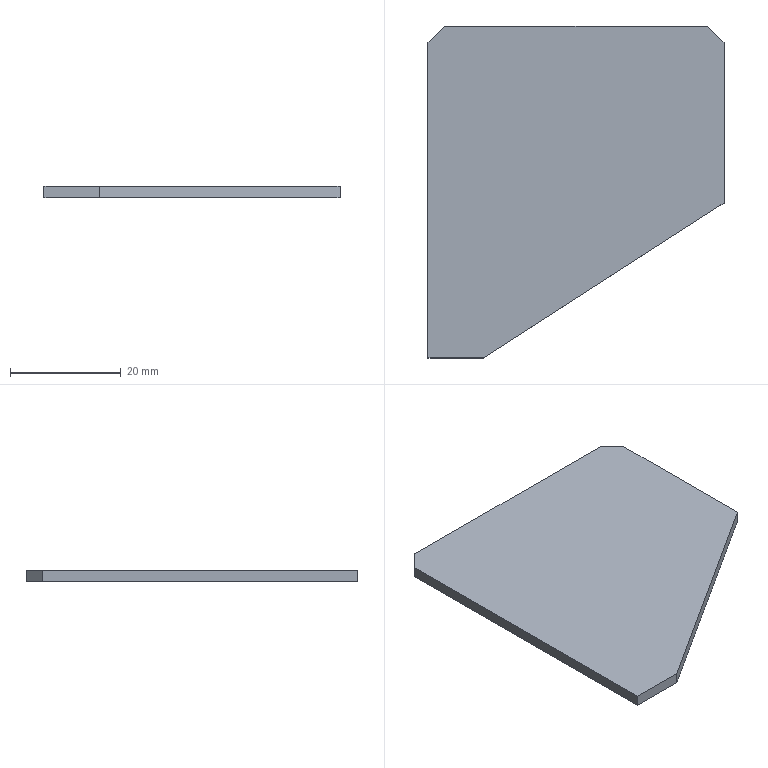Part | SolidWorks | features Chamfer 1, Extrusion 1 | 1 solid | 9 faces | box 53.5 x 60 x 2 mm | volume 5184 mm3 | plane 9
STEP:
#1=CARTESIAN_POINT('',(0.,-3.,2.));
#2=VERTEX_POINT('',#1);
#3=CARTESIAN_POINT('',(0.,-60.,2.));
#4=VERTEX_POINT('',#3);
#5=CARTESIAN_POINT('',(0.,-60.,2.));
#6=DIRECTION('',(0.,-1.,0.));
#7=VECTOR('',#6,1000.);
#8=LINE('',#5,#7);
#9=EDGE_CURVE('',#2,#4,#8,.T.);
#10=ORIENTED_EDGE('',*,*,#9,.F.);
#11=CARTESIAN_POINT('',(0.,-3.,0.));
#12=VERTEX_POINT('',#11);
#13=CARTESIAN_POINT('',(0.,-3.,2.));
#14=DIRECTION('',(0.,0.,-1.));
#15=VECTOR('',#14,1000.);
#16=LINE('',#13,#15);
#17=EDGE_CURVE('',#2,#12,#16,.T.);
#18=ORIENTED_EDGE('',*,*,#17,.T.);
#19=CARTESIAN_POINT('',(0.,-60.,0.));
#20=VERTEX_POINT('',#19);
#21=CARTESIAN_POINT('',(0.,-60.,0.));
#22=DIRECTION('',(0.,-1.,0.));
#23=VECTOR('',#22,1000.);
#24=LINE('',#21,#23);
#25=EDGE_CURVE('',#12,#20,#24,.T.);
#26=ORIENTED_EDGE('',*,*,#25,.T.);
#27=CARTESIAN_POINT('',(0.,-60.,2.));
#28=DIRECTION('',(0.,0.,-1.));
#29=VECTOR('',#28,1000.);
#30=LINE('',#27,#29);
#31=EDGE_CURVE('',#4,#20,#30,.T.);
#32=ORIENTED_EDGE('',*,*,#31,.F.);
#33=EDGE_LOOP('',(#10,#18,#26,#32));
#34=FACE_OUTER_BOUND('',#33,.T.);
#35=CARTESIAN_POINT('',(0.,-60.,2.));
#36=DIRECTION('',(1.,0.,0.));
#37=DIRECTION('',(0.,0.,-1.));
#38=AXIS2_PLACEMENT_3D('',#35,#36,#37);
#39=PLANE('',#38);
#40=ADVANCED_FACE('',(#34),#39,.F.);
#41=CARTESIAN_POINT('',(10.,-60.,0.));
#42=VERTEX_POINT('',#41);
#43=CARTESIAN_POINT('',(10.,-60.,0.));
#44=DIRECTION('',(1.,0.,0.));
#45=VECTOR('',#44,1000.);
#46=LINE('',#43,#45);
#47=EDGE_CURVE('',#20,#42,#46,.T.);
#48=ORIENTED_EDGE('',*,*,#47,.T.);
#49=CARTESIAN_POINT('',(10.,-60.,2.));
#50=VERTEX_POINT('',#49);
#51=CARTESIAN_POINT('',(10.,-60.,2.));
#52=DIRECTION('',(0.,0.,-1.));
#53=VECTOR('',#52,1000.);
#54=LINE('',#51,#53);
#55=EDGE_CURVE('',#50,#42,#54,.T.);
#56=ORIENTED_EDGE('',*,*,#55,.F.);
#57=CARTESIAN_POINT('',(10.,-60.,2.));
#58=DIRECTION('',(1.,0.,0.));
#59=VECTOR('',#58,1000.);
#60=LINE('',#57,#59);
#61=EDGE_CURVE('',#4,#50,#60,.T.);
#62=ORIENTED_EDGE('',*,*,#61,.F.);
#63=ORIENTED_EDGE('',*,*,#31,.T.);
#64=EDGE_LOOP('',(#48,#56,#62,#63));
#65=FACE_OUTER_BOUND('',#64,.T.);
#66=CARTESIAN_POINT('',(10.,-60.,2.));
#67=DIRECTION('',(0.,1.,0.));
#68=DIRECTION('',(0.,0.,1.));
#69=AXIS2_PLACEMENT_3D('',#66,#67,#68);
#70=PLANE('',#69);
#71=ADVANCED_FACE('',(#65),#70,.F.);
#72=CARTESIAN_POINT('',(53.5,-32.,0.));
#73=VERTEX_POINT('',#72);
#74=CARTESIAN_POINT('',(53.5,-32.,0.));
#75=DIRECTION('',(0.8409,0.5412,0.));
#76=VECTOR('',#75,1000.);
#77=LINE('',#74,#76);
#78=EDGE_CURVE('',#42,#73,#77,.T.);
#79=ORIENTED_EDGE('',*,*,#78,.T.);
#80=CARTESIAN_POINT('',(53.5,-32.,2.));
#81=VERTEX_POINT('',#80);
#82=CARTESIAN_POINT('',(53.5,-32.,2.));
#83=DIRECTION('',(0.,0.,-1.));
#84=VECTOR('',#83,1000.);
#85=LINE('',#82,#84);
#86=EDGE_CURVE('',#81,#73,#85,.T.);
#87=ORIENTED_EDGE('',*,*,#86,.F.);
#88=CARTESIAN_POINT('',(53.5,-32.,2.));
#89=DIRECTION('',(0.8409,0.5412,0.));
#90=VECTOR('',#89,1000.);
#91=LINE('',#88,#90);
#92=EDGE_CURVE('',#50,#81,#91,.T.);
#93=ORIENTED_EDGE('',*,*,#92,.F.);
#94=ORIENTED_EDGE('',*,*,#55,.T.);
#95=EDGE_LOOP('',(#79,#87,#93,#94));
#96=FACE_OUTER_BOUND('',#95,.T.);
#97=CARTESIAN_POINT('',(53.5,-32.,2.));
#98=DIRECTION('',(-0.5412,0.8409,0.));
#99=DIRECTION('',(-0.8409,-0.5412,0.));
#100=AXIS2_PLACEMENT_3D('',#97,#98,#99);
#101=PLANE('',#100);
#102=ADVANCED_FACE('',(#96),#101,.F.);
#103=CARTESIAN_POINT('',(53.5,-3.,0.));
#104=VERTEX_POINT('',#103);
#105=CARTESIAN_POINT('',(53.5,0.,0.));
#106=DIRECTION('',(0.,1.,0.));
#107=VECTOR('',#106,1000.);
#108=LINE('',#105,#107);
#109=EDGE_CURVE('',#73,#104,#108,.T.);
#110=ORIENTED_EDGE('',*,*,#109,.T.);
#111=CARTESIAN_POINT('',(53.5,-3.,2.));
#112=VERTEX_POINT('',#111);
#113=CARTESIAN_POINT('',(53.5,-3.,2.));
#114=DIRECTION('',(0.,0.,1.));
#115=VECTOR('',#114,1000.);
#116=LINE('',#113,#115);
#117=EDGE_CURVE('',#104,#112,#116,.T.);
#118=ORIENTED_EDGE('',*,*,#117,.T.);
#119=CARTESIAN_POINT('',(53.5,0.,2.));
#120=DIRECTION('',(0.,1.,0.));
#121=VECTOR('',#120,1000.);
#122=LINE('',#119,#121);
#123=EDGE_CURVE('',#81,#112,#122,.T.);
#124=ORIENTED_EDGE('',*,*,#123,.F.);
#125=ORIENTED_EDGE('',*,*,#86,.T.);
#126=EDGE_LOOP('',(#110,#118,#124,#125));
#127=FACE_OUTER_BOUND('',#126,.T.);
#128=CARTESIAN_POINT('',(53.5,0.,2.));
#129=DIRECTION('',(-1.,0.,0.));
#130=DIRECTION('',(0.,-1.,0.));
#131=AXIS2_PLACEMENT_3D('',#128,#129,#130);
#132=PLANE('',#131);
#133=ADVANCED_FACE('',(#127),#132,.F.);
#134=CARTESIAN_POINT('',(50.5,0.,2.));
#135=VERTEX_POINT('',#134);
#136=CARTESIAN_POINT('',(3.,0.,2.));
#137=VERTEX_POINT('',#136);
#138=CARTESIAN_POINT('',(0.,0.,2.));
#139=DIRECTION('',(-1.,0.,0.));
#140=VECTOR('',#139,1000.);
#141=LINE('',#138,#140);
#142=EDGE_CURVE('',#135,#137,#141,.T.);
#143=ORIENTED_EDGE('',*,*,#142,.F.);
#144=CARTESIAN_POINT('',(50.5,0.,0.));
#145=VERTEX_POINT('',#144);
#146=CARTESIAN_POINT('',(50.5,0.,2.));
#147=DIRECTION('',(0.,0.,-1.));
#148=VECTOR('',#147,1000.);
#149=LINE('',#146,#148);
#150=EDGE_CURVE('',#135,#145,#149,.T.);
#151=ORIENTED_EDGE('',*,*,#150,.T.);
#152=CARTESIAN_POINT('',(3.,0.,0.));
#153=VERTEX_POINT('',#152);
#154=CARTESIAN_POINT('',(0.,0.,0.));
#155=DIRECTION('',(-1.,0.,0.));
#156=VECTOR('',#155,1000.);
#157=LINE('',#154,#156);
#158=EDGE_CURVE('',#145,#153,#157,.T.);
#159=ORIENTED_EDGE('',*,*,#158,.T.);
#160=CARTESIAN_POINT('',(3.,0.,2.));
#161=DIRECTION('',(0.,0.,1.));
#162=VECTOR('',#161,1000.);
#163=LINE('',#160,#162);
#164=EDGE_CURVE('',#153,#137,#163,.T.);
#165=ORIENTED_EDGE('',*,*,#164,.T.);
#166=EDGE_LOOP('',(#143,#151,#159,#165));
#167=FACE_OUTER_BOUND('',#166,.T.);
#168=CARTESIAN_POINT('',(0.,0.,2.));
#169=DIRECTION('',(0.,-1.,0.));
#170=DIRECTION('',(0.,0.,-1.));
#171=AXIS2_PLACEMENT_3D('',#168,#169,#170);
#172=PLANE('',#171);
#173=ADVANCED_FACE('',(#167),#172,.F.);
#174=ORIENTED_EDGE('',*,*,#123,.T.);
#175=CARTESIAN_POINT('',(50.5,0.,2.));
#176=DIRECTION('',(-0.7071,0.7071,0.));
#177=VECTOR('',#176,1000.);
#178=LINE('',#175,#177);
#179=EDGE_CURVE('',#112,#135,#178,.T.);
#180=ORIENTED_EDGE('',*,*,#179,.T.);
#181=ORIENTED_EDGE('',*,*,#142,.T.);
#182=CARTESIAN_POINT('',(0.,-3.,2.));
#183=DIRECTION('',(-0.7071,-0.7071,0.));
#184=VECTOR('',#183,1000.);
#185=LINE('',#182,#184);
#186=EDGE_CURVE('',#137,#2,#185,.T.);
#187=ORIENTED_EDGE('',*,*,#186,.T.);
#188=ORIENTED_EDGE('',*,*,#9,.T.);
#189=ORIENTED_EDGE('',*,*,#61,.T.);
#190=ORIENTED_EDGE('',*,*,#92,.T.);
#191=EDGE_LOOP('',(#174,#180,#181,#187,#188,#189,#190));
#192=FACE_OUTER_BOUND('',#191,.T.);
#193=CARTESIAN_POINT('',(0.,0.,2.));
#194=DIRECTION('',(0.,0.,-1.));
#195=DIRECTION('',(-1.,0.,0.));
#196=AXIS2_PLACEMENT_3D('',#193,#194,#195);
#197=PLANE('',#196);
#198=ADVANCED_FACE('',(#192),#197,.F.);
#199=ORIENTED_EDGE('',*,*,#158,.F.);
#200=CARTESIAN_POINT('',(25.25,25.25,0.));
#201=DIRECTION('',(0.7071,-0.7071,0.));
#202=VECTOR('',#201,1000.);
#203=LINE('',#200,#202);
#204=EDGE_CURVE('',#145,#104,#203,.T.);
#205=ORIENTED_EDGE('',*,*,#204,.T.);
#206=ORIENTED_EDGE('',*,*,#109,.F.);
#207=ORIENTED_EDGE('',*,*,#78,.F.);
#208=ORIENTED_EDGE('',*,*,#47,.F.);
#209=ORIENTED_EDGE('',*,*,#25,.F.);
#210=CARTESIAN_POINT('',(1.5,-1.5,0.));
#211=DIRECTION('',(0.7071,0.7071,0.));
#212=VECTOR('',#211,1000.);
#213=LINE('',#210,#212);
#214=EDGE_CURVE('',#12,#153,#213,.T.);
#215=ORIENTED_EDGE('',*,*,#214,.T.);
#216=EDGE_LOOP('',(#199,#205,#206,#207,#208,#209,#215));
#217=FACE_OUTER_BOUND('',#216,.T.);
#218=CARTESIAN_POINT('',(0.,0.,0.));
#219=DIRECTION('',(0.,0.,-1.));
#220=DIRECTION('',(-1.,0.,0.));
#221=AXIS2_PLACEMENT_3D('',#218,#219,#220);
#222=PLANE('',#221);
#223=ADVANCED_FACE('',(#217),#222,.T.);
#224=ORIENTED_EDGE('',*,*,#179,.F.);
#225=ORIENTED_EDGE('',*,*,#117,.F.);
#226=ORIENTED_EDGE('',*,*,#204,.F.);
#227=ORIENTED_EDGE('',*,*,#150,.F.);
#228=EDGE_LOOP('',(#224,#225,#226,#227));
#229=FACE_OUTER_BOUND('',#228,.T.);
#230=CARTESIAN_POINT('',(50.5,0.,2.));
#231=DIRECTION('',(-0.7071,-0.7071,0.));
#232=DIRECTION('',(0.,0.,-1.));
#233=AXIS2_PLACEMENT_3D('',#230,#231,#232);
#234=PLANE('',#233);
#235=ADVANCED_FACE('',(#229),#234,.F.);
#236=ORIENTED_EDGE('',*,*,#186,.F.);
#237=ORIENTED_EDGE('',*,*,#164,.F.);
#238=ORIENTED_EDGE('',*,*,#214,.F.);
#239=ORIENTED_EDGE('',*,*,#17,.F.);
#240=EDGE_LOOP('',(#236,#237,#238,#239));
#241=FACE_OUTER_BOUND('',#240,.T.);
#242=CARTESIAN_POINT('',(0.,-3.,2.));
#243=DIRECTION('',(0.7071,-0.7071,0.));
#244=DIRECTION('',(0.,0.,-1.));
#245=AXIS2_PLACEMENT_3D('',#242,#243,#244);
#246=PLANE('',#245);
#247=ADVANCED_FACE('',(#241),#246,.F.);
#248=CLOSED_SHELL('',(#40,#71,#102,#133,#173,#198,#223,#235,#247));
#249=MANIFOLD_SOLID_BREP('',#248);
#250=CARTESIAN_POINT('',(0.,0.,0.));
#251=DIRECTION('',(0.,0.,1.));
#252=DIRECTION('',(1.,0.,0.));
#253=AXIS2_PLACEMENT_3D('',#250,#251,#252);
#254=(LENGTH_UNIT()NAMED_UNIT(*)SI_UNIT(.MILLI.,.METRE.));
#255=UNCERTAINTY_MEASURE_WITH_UNIT(LENGTH_MEASURE(0.00001),#254,'','');
#256=(NAMED_UNIT(*)PLANE_ANGLE_UNIT()SI_UNIT($,.RADIAN.));
#257=(NAMED_UNIT(*)SI_UNIT($,.STERADIAN.)SOLID_ANGLE_UNIT());
#258=(GEOMETRIC_REPRESENTATION_CONTEXT(3)GLOBAL_UNCERTAINTY_ASSIGNED_CONTEXT((#255))GLOBAL_UNIT_ASSIGNED_CONTEXT((#254,#256,#257))REPRESENTATION_CONTEXT('',''));
#259=ADVANCED_BREP_SHAPE_REPRESENTATION('',(#249,#253),#258);